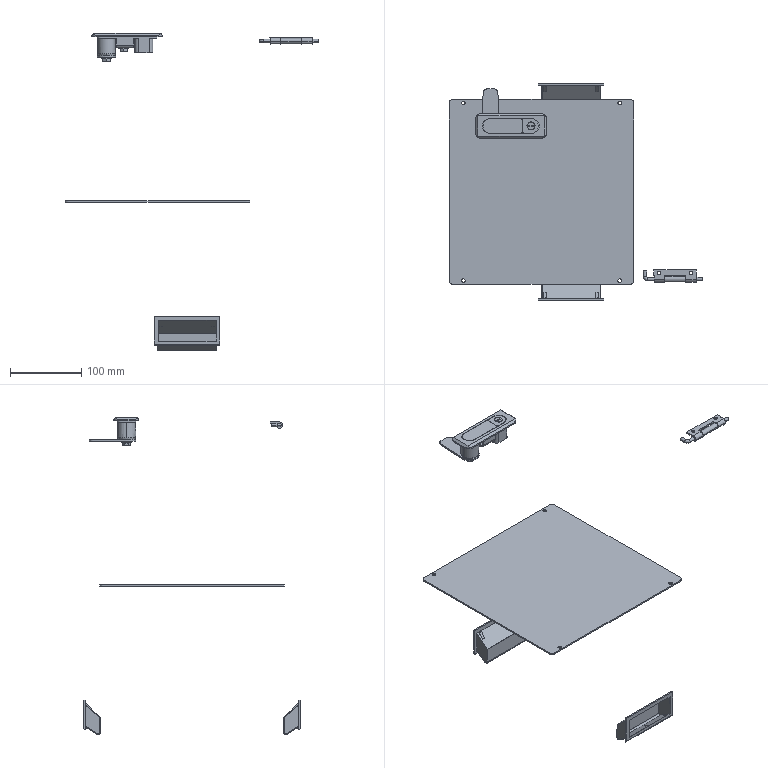Part | SolidWorks | features ReferencePattern 2, InContextFeatHolder 1, MirrorCompFeat 1 | 6 solids | 331 faces | box 356.977 x 304 x 446.493 mm | volume 211386 mm3 | plane 218 | cylinder 83 | cone 26 | torus 2 | spline 2 | commonest cylinder face diameters 5 x18 10 x14 4 x8 8 x8 9 x6 5.1 x4